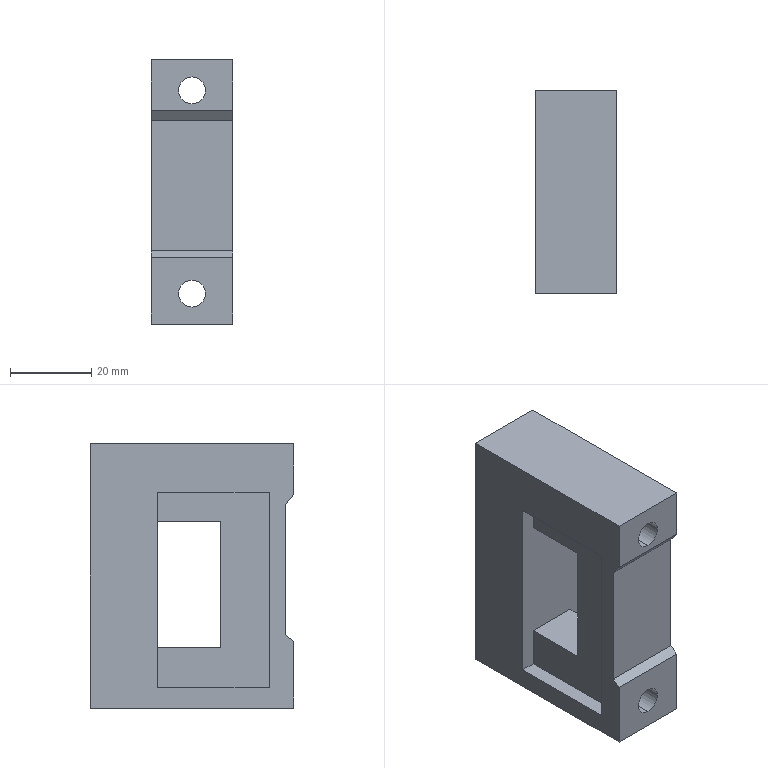Part | STEP file | Primary busbar bracket JTN1 | 1 solid | 40 faces | box 20 x 50 x 65 mm | volume 42874 mm3 | plane 30 | cylinder 10 | commonest cylinder face diameters 6.6 x4 11 x4 16 x2